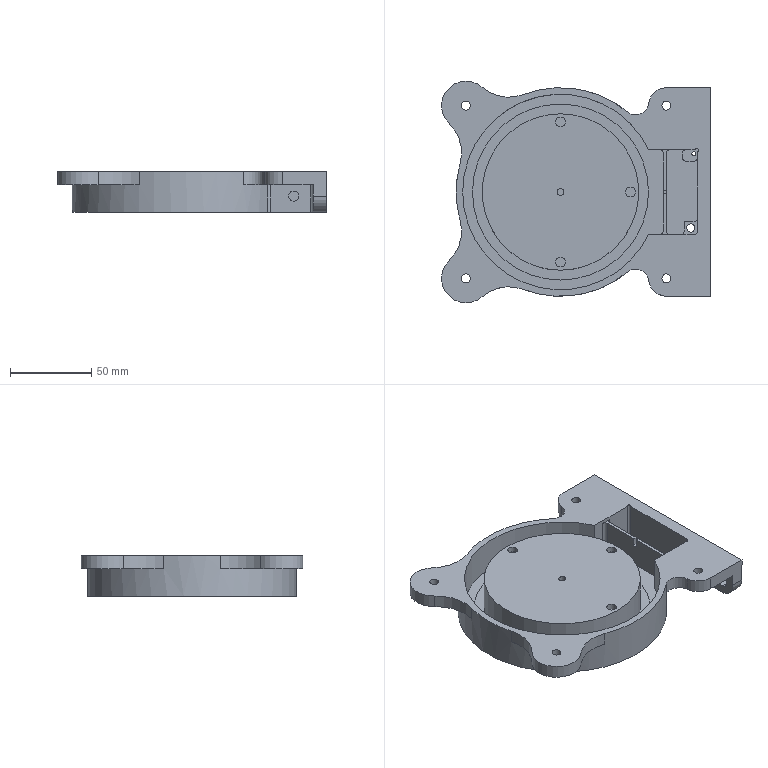NC program | NX | posted with a generic post | part box 165 x 136 x 25 mm
Lines 1 to 160 of 5148:
N10 G17 G21 G94 G90
(FLOOR_WALL_COPY , TOOL : D80)
N12 T08 M6
N14 G54
N16 G17 G0 G90 X-45. Y67.997 S6500 M3
N18 G43 Z30. H8
N20 Z7.51
N22 G94 G1 Z4.51 F1250.
N24 X-40.
N26 X205.
N28 Y15.999
N30 X-40.
N32 Y-36.
N34 X205.
N36 X210.
N38 Z7.51
N40 G0 Z30.
N42 X-45. Y67.997
N44 Z7.02
N46 G1 Z4.02
N48 X-40.
N50 X205.
N52 Y15.999
N54 X-40.
N56 Y-36.
N58 X205.
N60 X210.
N62 Z7.02
N64 G0 Z30.
N66 X-45. Y67.997
N68 Z6.53
N70 G1 Z3.53
N72 X-40.
N74 X205.
N76 Y15.999
N78 X-40.
N80 Y-36.
N82 X205.
N84 X210.
N86 Z6.53
N88 G0 Z30.
N90 X-45. Y67.997
N92 Z6.04
N94 G1 Z3.04
N96 X-40.
N98 X205.
N100 Y15.999
N102 X-40.
N104 Y-36.
N106 X205.
N108 X210.
N110 Z6.04
N112 G0 Z30.
N114 X-45. Y67.997
N116 Z5.55
N118 G1 Z2.55
N120 X-40.
N122 X205.
N124 Y15.999
N126 X-40.
N128 Y-36.
N130 X205.
N132 X210.
N134 Z5.55
N136 G0 Z30.
N138 X-45. Y67.997
N140 Z5.06
N142 G1 Z2.06
N144 X-40.
N146 X205.
N148 Y15.999
N150 X-40.
N152 Y-36.
N154 X205.
N156 X210.
N158 Z5.06
N160 G0 Z30.
N162 X-45. Y67.997
N164 Z4.57
N166 G1 Z1.57
N168 X-40.
N170 X205.
N172 Y15.999
N174 X-40.
N176 Y-36.
N178 X205.
N180 X210.
N182 Z4.57
N184 G0 Z30.
N186 X-45. Y67.997
N188 Z4.08
N190 G1 Z1.08
N192 X-40.
N194 X205.
N196 Y15.999
N198 X-40.
N200 Y-36.
N202 X205.
N204 X210.
N206 Z4.08
N208 G0 Z30.
N210 X-45. Y67.997
N212 Z3.59
N214 G1 Z0.59
N216 X-40.
N218 X205.
N220 Y15.999
N222 X-40.
N224 Y-36.
N226 X205.
N228 X210.
N230 Z3.59
N232 G0 Z30.
N234 X-45. Y67.997
N236 Z3.1
N238 G1 Z0.1
N240 X-40.
N242 X205.
N244 Y15.999
N246 X-40.
N248 Y-36.
N250 X205.
N252 X210.
N254 Z3.1
N256 G0 Z30.
(FACE_MILLING , TOOL : D80)
N258 X-80. Y0.
N260 Z3.
N262 G1 Z0.
N264 X-40.
N266 X196.
N268 X236.
N270 Z3.
N272 G0 Z30.
(PLANAR_MILL_1 , TOOL : D80)
N274 X256. Y-75.
N276 Z3.
N278 G1 Z0.
N280 X176.
N282 X-10.
N284 X-90.
N286 Z3.
N288 G0 Z30.
N290 X256. Y75.
N292 Z3.
N294 G1 Z0.
N296 X176.
N298 X-10.
N300 X-90.
N302 Z3.
N304 G0 Z30.
N306 M5